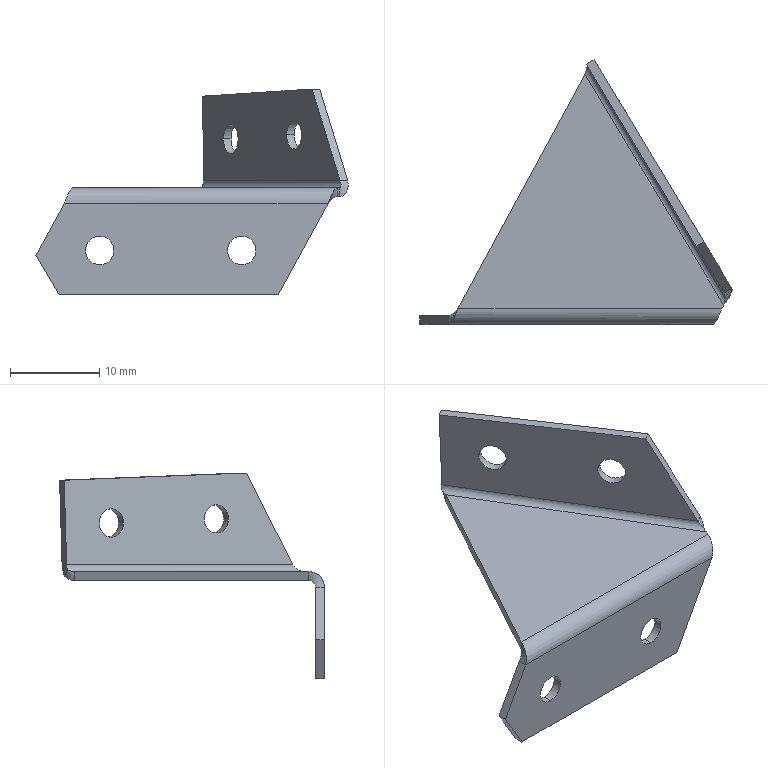Part | SolidWorks | features BaseBody 1 | 1 solid | 32 faces | box 35.031 x 29.701 x 23.105 mm | volume 1039 mm3 | plane 15 | cylinder 12 | spline 5 | commonest cylinder face diameters 3.2 x8 1.5 x2 3.5 x2
STEP:
#1=CARTESIAN_POINT('',(-8.394,13.485,6.933));
#2=VERTEX_POINT('',#1);
#3=CARTESIAN_POINT('',(-6.743,10.744,6.933));
#4=VERTEX_POINT('',#3);
#5=CARTESIAN_POINT('',(-7.568,12.114,6.933));
#6=DIRECTION('',(-0.8566,-0.516,0.));
#7=DIRECTION('',(-0.516,0.8566,0.));
#8=AXIS2_PLACEMENT_3D('',#5,#6,#7);
#9=CIRCLE('',#8,1.6);
#10=EDGE_CURVE('',#2,#4,#9,.T.);
#11=ORIENTED_EDGE('',*,*,#10,.T.);
#12=CARTESIAN_POINT('',(-5.886,11.26,6.933));
#13=VERTEX_POINT('',#12);
#14=CARTESIAN_POINT('',(-6.743,10.744,6.933));
#15=DIRECTION('',(0.8566,0.516,0.));
#16=VECTOR('',#15,1000.);
#17=LINE('',#14,#16);
#18=EDGE_CURVE('',#4,#13,#17,.T.);
#19=ORIENTED_EDGE('',*,*,#18,.T.);
#20=CARTESIAN_POINT('',(-7.537,14.001,6.933));
#21=VERTEX_POINT('',#20);
#22=CARTESIAN_POINT('',(-6.712,12.63,6.933));
#23=DIRECTION('',(0.8566,0.516,0.));
#24=DIRECTION('',(-0.516,0.8566,0.));
#25=AXIS2_PLACEMENT_3D('',#22,#23,#24);
#26=CIRCLE('',#25,1.6);
#27=EDGE_CURVE('',#13,#21,#26,.T.);
#28=ORIENTED_EDGE('',*,*,#27,.T.);
#29=CARTESIAN_POINT('',(-8.394,13.485,6.933));
#30=DIRECTION('',(0.8566,0.516,0.));
#31=VECTOR('',#30,1000.);
#32=LINE('',#29,#31);
#33=EDGE_CURVE('',#2,#21,#32,.T.);
#34=ORIENTED_EDGE('',*,*,#33,.F.);
#35=EDGE_LOOP('',(#11,#19,#28,#34));
#36=FACE_OUTER_BOUND('',#35,.T.);
#37=CARTESIAN_POINT('',(-7.568,12.114,6.933));
#38=DIRECTION('',(0.8566,0.516,0.));
#39=DIRECTION('',(-0.516,0.8566,0.));
#40=AXIS2_PLACEMENT_3D('',#37,#38,#39);
#41=CYLINDRICAL_SURFACE('',#40,1.6);
#42=ADVANCED_FACE('',(#36),#41,.F.);
#43=CARTESIAN_POINT('',(-15.496,25.274,6.468));
#44=VERTEX_POINT('',#43);
#45=CARTESIAN_POINT('',(-13.845,22.533,6.468));
#46=VERTEX_POINT('',#45);
#47=CARTESIAN_POINT('',(-14.671,23.904,6.468));
#48=DIRECTION('',(-0.8566,-0.516,0.));
#49=DIRECTION('',(-0.516,0.8566,0.));
#50=AXIS2_PLACEMENT_3D('',#47,#48,#49);
#51=CIRCLE('',#50,1.6);
#52=EDGE_CURVE('',#44,#46,#51,.T.);
#53=ORIENTED_EDGE('',*,*,#52,.T.);
#54=CARTESIAN_POINT('',(-12.988,23.049,6.468));
#55=VERTEX_POINT('',#54);
#56=CARTESIAN_POINT('',(-13.845,22.533,6.468));
#57=DIRECTION('',(0.8566,0.516,0.));
#58=VECTOR('',#57,1000.);
#59=LINE('',#56,#58);
#60=EDGE_CURVE('',#46,#55,#59,.T.);
#61=ORIENTED_EDGE('',*,*,#60,.T.);
#62=CARTESIAN_POINT('',(-14.64,25.79,6.468));
#63=VERTEX_POINT('',#62);
#64=CARTESIAN_POINT('',(-13.814,24.42,6.468));
#65=DIRECTION('',(-0.8566,-0.516,0.));
#66=DIRECTION('',(-0.516,0.8566,0.));
#67=AXIS2_PLACEMENT_3D('',#64,#65,#66);
#68=CIRCLE('',#67,1.6);
#69=EDGE_CURVE('',#63,#55,#68,.T.);
#70=ORIENTED_EDGE('',*,*,#69,.F.);
#71=CARTESIAN_POINT('',(-15.496,25.274,6.468));
#72=DIRECTION('',(0.8566,0.516,0.));
#73=VECTOR('',#72,1000.);
#74=LINE('',#71,#73);
#75=EDGE_CURVE('',#44,#63,#74,.T.);
#76=ORIENTED_EDGE('',*,*,#75,.F.);
#77=EDGE_LOOP('',(#53,#61,#70,#76));
#78=FACE_OUTER_BOUND('',#77,.T.);
#79=CARTESIAN_POINT('',(-14.671,23.904,6.468));
#80=DIRECTION('',(0.8566,0.516,0.));
#81=DIRECTION('',(-0.516,0.8566,0.));
#82=AXIS2_PLACEMENT_3D('',#79,#80,#81);
#83=CYLINDRICAL_SURFACE('',#82,1.6);
#84=ADVANCED_FACE('',(#78),#83,.F.);
#85=CARTESIAN_POINT('',(-29.376,0.,-4.437));
#86=VERTEX_POINT('',#85);
#87=CARTESIAN_POINT('',(-29.376,0.,-7.637));
#88=VERTEX_POINT('',#87);
#89=CARTESIAN_POINT('',(-29.376,0.,-6.037));
#90=DIRECTION('',(0.,-1.,0.));
#91=DIRECTION('',(0.,0.,1.));
#92=AXIS2_PLACEMENT_3D('',#89,#90,#91);
#93=CIRCLE('',#92,1.6);
#94=EDGE_CURVE('',#86,#88,#93,.T.);
#95=ORIENTED_EDGE('',*,*,#94,.T.);
#96=CARTESIAN_POINT('',(-29.376,1.,-7.637));
#97=VERTEX_POINT('',#96);
#98=CARTESIAN_POINT('',(-29.376,0.,-7.637));
#99=DIRECTION('',(0.,1.,0.));
#100=VECTOR('',#99,1000.);
#101=LINE('',#98,#100);
#102=EDGE_CURVE('',#88,#97,#101,.T.);
#103=ORIENTED_EDGE('',*,*,#102,.T.);
#104=CARTESIAN_POINT('',(-29.376,1.,-4.437));
#105=VERTEX_POINT('',#104);
#106=CARTESIAN_POINT('',(-29.376,1.,-6.037));
#107=DIRECTION('',(0.,-1.,0.));
#108=DIRECTION('',(0.,0.,1.));
#109=AXIS2_PLACEMENT_3D('',#106,#107,#108);
#110=CIRCLE('',#109,1.6);
#111=EDGE_CURVE('',#105,#97,#110,.T.);
#112=ORIENTED_EDGE('',*,*,#111,.F.);
#113=CARTESIAN_POINT('',(-29.376,0.,-4.437));
#114=DIRECTION('',(0.,1.,0.));
#115=VECTOR('',#114,1000.);
#116=LINE('',#113,#115);
#117=EDGE_CURVE('',#86,#105,#116,.T.);
#118=ORIENTED_EDGE('',*,*,#117,.F.);
#119=EDGE_LOOP('',(#95,#103,#112,#118));
#120=FACE_OUTER_BOUND('',#119,.T.);
#121=CARTESIAN_POINT('',(-29.376,0.,-6.037));
#122=DIRECTION('',(0.,1.,0.));
#123=DIRECTION('',(0.,0.,1.));
#124=AXIS2_PLACEMENT_3D('',#121,#122,#123);
#125=CYLINDRICAL_SURFACE('',#124,1.6);
#126=ADVANCED_FACE('',(#120),#125,.F.);
#127=CARTESIAN_POINT('',(-13.445,0.,-4.437));
#128=VERTEX_POINT('',#127);
#129=CARTESIAN_POINT('',(-13.445,0.,-7.637));
#130=VERTEX_POINT('',#129);
#131=CARTESIAN_POINT('',(-13.445,0.,-6.037));
#132=DIRECTION('',(0.,-1.,0.));
#133=DIRECTION('',(0.,0.,1.));
#134=AXIS2_PLACEMENT_3D('',#131,#132,#133);
#135=CIRCLE('',#134,1.6);
#136=EDGE_CURVE('',#128,#130,#135,.T.);
#137=ORIENTED_EDGE('',*,*,#136,.T.);
#138=CARTESIAN_POINT('',(-13.445,1.,-7.637));
#139=VERTEX_POINT('',#138);
#140=CARTESIAN_POINT('',(-13.445,0.,-7.637));
#141=DIRECTION('',(0.,1.,0.));
#142=VECTOR('',#141,1000.);
#143=LINE('',#140,#142);
#144=EDGE_CURVE('',#130,#139,#143,.T.);
#145=ORIENTED_EDGE('',*,*,#144,.T.);
#146=CARTESIAN_POINT('',(-13.445,1.,-4.437));
#147=VERTEX_POINT('',#146);
#148=CARTESIAN_POINT('',(-13.445,1.,-6.037));
#149=DIRECTION('',(0.,-1.,0.));
#150=DIRECTION('',(0.,0.,1.));
#151=AXIS2_PLACEMENT_3D('',#148,#149,#150);
#152=CIRCLE('',#151,1.6);
#153=EDGE_CURVE('',#147,#139,#152,.T.);
#154=ORIENTED_EDGE('',*,*,#153,.F.);
#155=CARTESIAN_POINT('',(-13.445,0.,-4.437));
#156=DIRECTION('',(0.,1.,0.));
#157=VECTOR('',#156,1000.);
#158=LINE('',#155,#157);
#159=EDGE_CURVE('',#128,#147,#158,.T.);
#160=ORIENTED_EDGE('',*,*,#159,.F.);
#161=EDGE_LOOP('',(#137,#145,#154,#160));
#162=FACE_OUTER_BOUND('',#161,.T.);
#163=CARTESIAN_POINT('',(-13.445,0.,-6.037));
#164=DIRECTION('',(0.,1.,0.));
#165=DIRECTION('',(0.,0.,1.));
#166=AXIS2_PLACEMENT_3D('',#163,#164,#165);
#167=CYLINDRICAL_SURFACE('',#166,1.6);
#168=ADVANCED_FACE('',(#162),#167,.F.);
#169=ORIENTED_EDGE('',*,*,#18,.F.);
#170=CARTESIAN_POINT('',(-7.568,12.114,6.933));
#171=DIRECTION('',(-0.8566,-0.516,0.));
#172=DIRECTION('',(-0.516,0.8566,0.));
#173=AXIS2_PLACEMENT_3D('',#170,#171,#172);
#174=CIRCLE('',#173,1.6);
#175=EDGE_CURVE('',#4,#2,#174,.T.);
#176=ORIENTED_EDGE('',*,*,#175,.T.);
#177=ORIENTED_EDGE('',*,*,#33,.T.);
#178=CARTESIAN_POINT('',(-6.712,12.63,6.933));
#179=DIRECTION('',(0.8566,0.516,0.));
#180=DIRECTION('',(-0.516,0.8566,0.));
#181=AXIS2_PLACEMENT_3D('',#178,#179,#180);
#182=CIRCLE('',#181,1.6);
#183=EDGE_CURVE('',#21,#13,#182,.T.);
#184=ORIENTED_EDGE('',*,*,#183,.T.);
#185=EDGE_LOOP('',(#169,#176,#177,#184));
#186=FACE_OUTER_BOUND('',#185,.T.);
#187=CARTESIAN_POINT('',(-7.568,12.114,6.933));
#188=DIRECTION('',(0.8566,0.516,0.));
#189=DIRECTION('',(-0.516,0.8566,0.));
#190=AXIS2_PLACEMENT_3D('',#187,#188,#189);
#191=CYLINDRICAL_SURFACE('',#190,1.6);
#192=ADVANCED_FACE('',(#186),#191,.F.);
#193=ORIENTED_EDGE('',*,*,#69,.T.);
#194=CARTESIAN_POINT('',(-13.814,24.42,6.468));
#195=DIRECTION('',(-0.8566,-0.516,0.));
#196=DIRECTION('',(-0.516,0.8566,0.));
#197=AXIS2_PLACEMENT_3D('',#194,#195,#196);
#198=CIRCLE('',#197,1.6);
#199=EDGE_CURVE('',#55,#63,#198,.T.);
#200=ORIENTED_EDGE('',*,*,#199,.T.);
#201=EDGE_LOOP('',(#193,#200));
#202=FACE_BOUND('',#201,.T.);
#203=ORIENTED_EDGE('',*,*,#183,.F.);
#204=ORIENTED_EDGE('',*,*,#27,.F.);
#205=EDGE_LOOP('',(#203,#204));
#206=FACE_BOUND('',#205,.T.);
#207=CARTESIAN_POINT('',(-16.995,29.701,11.262));
#208=VERTEX_POINT('',#207);
#209=CARTESIAN_POINT('',(-4.678,9.254,12.069));
#210=VERTEX_POINT('',#209);
#211=CARTESIAN_POINT('',(-16.995,29.701,11.262));
#212=DIRECTION('',(0.5157,-0.8561,0.03376));
#213=VECTOR('',#212,1000.);
#214=LINE('',#211,#213);
#215=EDGE_CURVE('',#208,#210,#214,.T.);
#216=ORIENTED_EDGE('',*,*,#215,.T.);
#217=CARTESIAN_POINT('',(-1.55,4.061,1.75));
#218=VERTEX_POINT('',#217);
#219=CARTESIAN_POINT('',(-4.678,9.254,12.069));
#220=DIRECTION('',(0.2614,-0.4339,-0.8622));
#221=VECTOR('',#220,1000.);
#222=LINE('',#219,#221);
#223=EDGE_CURVE('',#210,#218,#222,.T.);
#224=ORIENTED_EDGE('',*,*,#223,.T.);
#225=CARTESIAN_POINT('',(-16.83,29.426,1.75));
#226=VERTEX_POINT('',#225);
#227=CARTESIAN_POINT('',(-1.55,4.061,1.75));
#228=DIRECTION('',(-0.516,0.8566,0.));
#229=VECTOR('',#228,1000.);
#230=LINE('',#227,#229);
#231=EDGE_CURVE('',#218,#226,#230,.T.);
#232=ORIENTED_EDGE('',*,*,#231,.T.);
#233=CARTESIAN_POINT('',(-16.83,29.426,1.75));
#234=DIRECTION('',(-0.01742,0.02892,0.9994));
#235=VECTOR('',#234,1000.);
#236=LINE('',#233,#235);
#237=EDGE_CURVE('',#226,#208,#236,.T.);
#238=ORIENTED_EDGE('',*,*,#237,.T.);
#239=EDGE_LOOP('',(#216,#224,#232,#238));
#240=FACE_OUTER_BOUND('',#239,.T.);
#241=CARTESIAN_POINT('',(-19.235,33.419,4.412));
#242=DIRECTION('',(0.8566,0.516,0.));
#243=DIRECTION('',(0.2663,-0.442,0.8566));
#244=AXIS2_PLACEMENT_3D('',#241,#242,#243);
#245=PLANE('',#244);
#246=ADVANCED_FACE('',(#202,#206,#240),#245,.T.);
#247=ORIENTED_EDGE('',*,*,#52,.F.);
#248=CARTESIAN_POINT('',(-14.671,23.904,6.468));
#249=DIRECTION('',(-0.8566,-0.516,0.));
#250=DIRECTION('',(-0.516,0.8566,0.));
#251=AXIS2_PLACEMENT_3D('',#248,#249,#250);
#252=CIRCLE('',#251,1.6);
#253=EDGE_CURVE('',#46,#44,#252,.T.);
#254=ORIENTED_EDGE('',*,*,#253,.F.);
#255=EDGE_LOOP('',(#247,#254));
#256=FACE_BOUND('',#255,.T.);
#257=ORIENTED_EDGE('',*,*,#10,.F.);
#258=ORIENTED_EDGE('',*,*,#175,.F.);
#259=EDGE_LOOP('',(#257,#258));
#260=FACE_BOUND('',#259,.T.);
#261=CARTESIAN_POINT('',(-17.852,29.185,11.262));
#262=VERTEX_POINT('',#261);
#263=CARTESIAN_POINT('',(-5.534,8.738,12.069));
#264=VERTEX_POINT('',#263);
#265=CARTESIAN_POINT('',(-5.534,8.738,12.069));
#266=DIRECTION('',(0.5157,-0.8561,0.03376));
#267=VECTOR('',#266,1000.);
#268=LINE('',#265,#267);
#269=EDGE_CURVE('',#262,#264,#268,.T.);
#270=ORIENTED_EDGE('',*,*,#269,.F.);
#271=CARTESIAN_POINT('',(-17.686,28.91,1.75));
#272=VERTEX_POINT('',#271);
#273=CARTESIAN_POINT('',(-17.852,29.185,11.262));
#274=DIRECTION('',(-0.01742,0.02892,0.9994));
#275=VECTOR('',#274,1000.);
#276=LINE('',#273,#275);
#277=EDGE_CURVE('',#272,#262,#276,.T.);
#278=ORIENTED_EDGE('',*,*,#277,.F.);
#279=CARTESIAN_POINT('',(-2.406,3.545,1.75));
#280=VERTEX_POINT('',#279);
#281=CARTESIAN_POINT('',(-17.782,29.068,1.75));
#282=DIRECTION('',(-0.516,0.8566,0.));
#283=VECTOR('',#282,1000.);
#284=LINE('',#281,#283);
#285=EDGE_CURVE('',#280,#272,#284,.T.);
#286=ORIENTED_EDGE('',*,*,#285,.F.);
#287=CARTESIAN_POINT('',(-2.406,3.545,1.75));
#288=DIRECTION('',(0.2614,-0.4339,-0.8622));
#289=VECTOR('',#288,1000.);
#290=LINE('',#287,#289);
#291=EDGE_CURVE('',#264,#280,#290,.T.);
#292=ORIENTED_EDGE('',*,*,#291,.F.);
#293=EDGE_LOOP('',(#270,#278,#286,#292));
#294=FACE_OUTER_BOUND('',#293,.T.);
#295=CARTESIAN_POINT('',(-20.092,32.903,4.412));
#296=DIRECTION('',(0.8566,0.516,0.));
#297=DIRECTION('',(0.2663,-0.442,0.8566));
#298=AXIS2_PLACEMENT_3D('',#295,#296,#297);
#299=PLANE('',#298);
#300=ADVANCED_FACE('',(#256,#260,#294),#299,.F.);
#301=ORIENTED_EDGE('',*,*,#60,.F.);
#302=ORIENTED_EDGE('',*,*,#253,.T.);
#303=ORIENTED_EDGE('',*,*,#75,.T.);
#304=ORIENTED_EDGE('',*,*,#199,.F.);
#305=EDGE_LOOP('',(#301,#302,#303,#304));
#306=FACE_OUTER_BOUND('',#305,.T.);
#307=CARTESIAN_POINT('',(-14.671,23.904,6.468));
#308=DIRECTION('',(0.8566,0.516,0.));
#309=DIRECTION('',(-0.516,0.8566,0.));
#310=AXIS2_PLACEMENT_3D('',#307,#308,#309);
#311=CYLINDRICAL_SURFACE('',#310,1.6);
#312=ADVANCED_FACE('',(#306),#311,.F.);
#313=CARTESIAN_POINT('',(-5.106,8.996,12.069));
#314=DIRECTION('',(-0.8566,-0.516,0.));
#315=VECTOR('',#314,1000.);
#316=LINE('',#313,#315);
#317=EDGE_CURVE('',#210,#264,#316,.T.);
#318=ORIENTED_EDGE('',*,*,#317,.T.);
#319=ORIENTED_EDGE('',*,*,#291,.T.);
#320=CARTESIAN_POINT('',(-1.978,3.803,1.75));
#321=DIRECTION('',(-0.8566,-0.516,0.));
#322=VECTOR('',#321,1000.);
#323=LINE('',#320,#322);
#324=EDGE_CURVE('',#218,#280,#323,.T.);
#325=ORIENTED_EDGE('',*,*,#324,.F.);
#326=ORIENTED_EDGE('',*,*,#223,.F.);
#327=EDGE_LOOP('',(#318,#319,#325,#326));
#328=FACE_OUTER_BOUND('',#327,.T.);
#329=CARTESIAN_POINT('',(-1.55,4.061,1.75));
#330=DIRECTION('',(0.4449,-0.7385,0.5066));
#331=DIRECTION('',(-0.2614,0.4339,0.8622));
#332=AXIS2_PLACEMENT_3D('',#329,#330,#331);
#333=PLANE('',#332);
#334=ADVANCED_FACE('',(#328),#333,.T.);
#335=ORIENTED_EDGE('',*,*,#269,.T.);
#336=ORIENTED_EDGE('',*,*,#317,.F.);
#337=ORIENTED_EDGE('',*,*,#215,.F.);
#338=CARTESIAN_POINT('',(-17.424,29.443,11.262));
#339=DIRECTION('',(-0.8566,-0.516,0.));
#340=VECTOR('',#339,1000.);
#341=LINE('',#338,#340);
#342=EDGE_CURVE('',#208,#262,#341,.T.);
#343=ORIENTED_EDGE('',*,*,#342,.T.);
#344=EDGE_LOOP('',(#335,#336,#337,#343));
#345=FACE_OUTER_BOUND('',#344,.T.);
#346=CARTESIAN_POINT('',(-4.678,9.254,12.069));
#347=DIRECTION('',(-0.01742,0.02892,0.9994));
#348=DIRECTION('',(-0.5157,0.8561,-0.03376));
#349=AXIS2_PLACEMENT_3D('',#346,#347,#348);
#350=PLANE('',#349);
#351=ADVANCED_FACE('',(#345),#350,.T.);
#352=ORIENTED_EDGE('',*,*,#342,.F.);
#353=ORIENTED_EDGE('',*,*,#237,.F.);
#354=CARTESIAN_POINT('',(-17.258,29.168,1.75));
#355=DIRECTION('',(-0.8566,-0.516,0.));
#356=VECTOR('',#355,1000.);
#357=LINE('',#354,#356);
#358=EDGE_CURVE('',#226,#272,#357,.T.);
#359=ORIENTED_EDGE('',*,*,#358,.T.);
#360=ORIENTED_EDGE('',*,*,#277,.T.);
#361=EDGE_LOOP('',(#352,#353,#359,#360));
#362=FACE_OUTER_BOUND('',#361,.T.);
#363=CARTESIAN_POINT('',(-16.995,29.701,11.262));
#364=DIRECTION('',(-0.5157,0.8561,-0.03376));
#365=DIRECTION('',(0.01742,-0.02892,-0.9994));
#366=AXIS2_PLACEMENT_3D('',#363,#364,#365);
#367=PLANE('',#366);
#368=ADVANCED_FACE('',(#362),#367,.T.);
#369=ORIENTED_EDGE('',*,*,#231,.F.);
#370=CARTESIAN_POINT('',(-2.453,2.17,0.));
#371=VERTEX_POINT('',#370);
#372=CARTESIAN_POINT('',(-2.453,2.17,0.));
#373=CARTESIAN_POINT('',(-2.305,2.372,0.));
#374=CARTESIAN_POINT('',(-2.161,2.57,0.04509));
#375=CARTESIAN_POINT('',(-1.962,2.859,0.1772));
#376=CARTESIAN_POINT('',(-1.901,2.952,0.2311));
#377=CARTESIAN_POINT('',(-1.788,3.131,0.3577));
#378=CARTESIAN_POINT('',(-1.736,3.219,0.4312));
#379=CARTESIAN_POINT('',(-1.647,3.386,0.5935));
#380=CARTESIAN_POINT('',(-1.609,3.464,0.6817));
#381=CARTESIAN_POINT('',(-1.55,3.611,0.8714));
#382=CARTESIAN_POINT('',(-1.528,3.681,0.974));
#383=CARTESIAN_POINT('',(-1.489,3.873,1.291));
#384=CARTESIAN_POINT('',(-1.5,3.978,1.519));
#385=CARTESIAN_POINT('',(-1.55,4.061,1.75));
#386=B_SPLINE_CURVE_WITH_KNOTS('',3,(#372,#373,#374,#375,#376,#377,#378,#379,#380,#381,#382,#383,#384,#385),.UNSPECIFIED.,.F.,.F.,(4,2,2,2,2,2,4),(0.,0.0007413,0.001112,0.001483,0.001853,0.002224,0.002965),.UNSPECIFIED.);
#387=EDGE_CURVE('',#371,#218,#386,.T.);
#388=ORIENTED_EDGE('',*,*,#387,.F.);
#389=CARTESIAN_POINT('',(-18.014,28.,0.));
#390=VERTEX_POINT('',#389);
#391=CARTESIAN_POINT('',(-10.391,15.346,0.));
#392=DIRECTION('',(0.516,-0.8566,0.));
#393=VECTOR('',#392,1000.);
#394=LINE('',#391,#393);
#395=EDGE_CURVE('',#390,#371,#394,.T.);
#396=ORIENTED_EDGE('',*,*,#395,.F.);
#397=CARTESIAN_POINT('',(-17.252,29.133,0.5126));
#398=VERTEX_POINT('',#397);
#399=CARTESIAN_POINT('',(-17.252,29.133,0.5126));
#400=CARTESIAN_POINT('',(-17.342,28.965,0.3491));
#401=CARTESIAN_POINT('',(-17.457,28.785,0.2214));
#402=CARTESIAN_POINT('',(-17.721,28.4,0.04513));
#403=CARTESIAN_POINT('',(-17.866,28.203,0.));
#404=CARTESIAN_POINT('',(-18.014,28.,0.));
#405=B_SPLINE_CURVE_WITH_KNOTS('',3,(#399,#400,#401,#402,#403,#404),.UNSPECIFIED.,.F.,.F.,(4,2,4),(0.,0.0007413,0.001483),.UNSPECIFIED.);
#406=EDGE_CURVE('',#398,#390,#405,.T.);
#407=ORIENTED_EDGE('',*,*,#406,.F.);
#408=CARTESIAN_POINT('',(-16.83,29.426,1.75));
#409=CARTESIAN_POINT('',(-16.827,29.421,1.521));
#410=CARTESIAN_POINT('',(-16.863,29.393,1.292));
#411=CARTESIAN_POINT('',(-17.007,29.293,0.8687));
#412=CARTESIAN_POINT('',(-17.116,29.221,0.6745));
#413=CARTESIAN_POINT('',(-17.252,29.133,0.5126));
#414=B_SPLINE_CURVE_WITH_KNOTS('',3,(#408,#409,#410,#411,#412,#413),.UNSPECIFIED.,.F.,.F.,(4,2,4),(0.,0.5,1.),.UNSPECIFIED.);
#415=EDGE_CURVE('',#226,#398,#414,.T.);
#416=ORIENTED_EDGE('',*,*,#415,.F.);
#417=EDGE_LOOP('',(#369,#388,#396,#407,#416));
#418=FACE_OUTER_BOUND('',#417,.T.);
#419=CARTESIAN_POINT('',(-18.424,28.681,1.75));
#420=DIRECTION('',(0.516,-0.8566,0.));
#421=DIRECTION('',(0.8566,0.516,0.));
#422=AXIS2_PLACEMENT_3D('',#419,#420,#421);
#423=CYLINDRICAL_SURFACE('',#422,1.75);
#424=ADVANCED_FACE('',(#418),#423,.T.);
#425=CARTESIAN_POINT('',(-2.453,2.17,1.));
#426=VERTEX_POINT('',#425);
#427=CARTESIAN_POINT('',(-2.453,2.17,1.));
#428=CARTESIAN_POINT('',(-2.419,2.304,1.));
#429=CARTESIAN_POINT('',(-2.385,2.435,1.019));
#430=CARTESIAN_POINT('',(-2.328,2.694,1.094));
#431=CARTESIAN_POINT('',(-2.307,2.819,1.15));
#432=CARTESIAN_POINT('',(-2.287,3.055,1.288));
#433=CARTESIAN_POINT('',(-2.289,3.167,1.372));
#434=CARTESIAN_POINT('',(-2.323,3.369,1.553));
#435=CARTESIAN_POINT('',(-2.356,3.462,1.651));
#436=CARTESIAN_POINT('',(-2.406,3.545,1.75));
#437=B_SPLINE_CURVE_WITH_KNOTS('',3,(#427,#428,#429,#430,#431,#432,#433,#434,#435,#436),.UNSPECIFIED.,.F.,.F.,(4,2,2,2,4),(0.,0.0004099,0.0008199,0.00123,0.00164),.UNSPECIFIED.);
#438=EDGE_CURVE('',#426,#280,#437,.T.);
#439=ORIENTED_EDGE('',*,*,#438,.T.);
#440=ORIENTED_EDGE('',*,*,#285,.T.);
#441=CARTESIAN_POINT('',(-17.857,28.768,1.22));
#442=VERTEX_POINT('',#441);
#443=CARTESIAN_POINT('',(-17.686,28.91,1.75));
#444=CARTESIAN_POINT('',(-17.681,28.9,1.554));
#445=CARTESIAN_POINT('',(-17.744,28.849,1.359));
#446=CARTESIAN_POINT('',(-17.857,28.768,1.22));
#447=B_SPLINE_CURVE_WITH_KNOTS('',3,(#443,#444,#445,#446),.UNSPECIFIED.,.F.,.F.,(4,4),(0.,1.),.UNSPECIFIED.);
#448=EDGE_CURVE('',#272,#442,#447,.T.);
#449=ORIENTED_EDGE('',*,*,#448,.T.);
#450=CARTESIAN_POINT('',(-18.014,28.,1.));
#451=VERTEX_POINT('',#450);
#452=CARTESIAN_POINT('',(-17.857,28.768,1.22));
#453=CARTESIAN_POINT('',(-17.877,28.531,1.08));
#454=CARTESIAN_POINT('',(-17.945,28.267,1.));
#455=CARTESIAN_POINT('',(-18.014,28.,1.));
#456=B_SPLINE_CURVE_WITH_KNOTS('',3,(#452,#453,#454,#455),.UNSPECIFIED.,.F.,.F.,(4,4),(0.,0.0008241),.UNSPECIFIED.);
#457=EDGE_CURVE('',#442,#451,#456,.T.);
#458=ORIENTED_EDGE('',*,*,#457,.T.);
#459=CARTESIAN_POINT('',(-10.391,15.346,1.));
#460=DIRECTION('',(0.516,-0.8566,0.));
#461=VECTOR('',#460,1000.);
#462=LINE('',#459,#461);
#463=EDGE_CURVE('',#451,#426,#462,.T.);
#464=ORIENTED_EDGE('',*,*,#463,.T.);
#465=EDGE_LOOP('',(#439,#440,#449,#458,#464));
#466=FACE_OUTER_BOUND('',#465,.T.);
#467=CARTESIAN_POINT('',(-18.424,28.681,1.75));
#468=DIRECTION('',(0.516,-0.8566,0.));
#469=DIRECTION('',(0.8566,0.516,0.));
#470=AXIS2_PLACEMENT_3D('',#467,#468,#469);
#471=CYLINDRICAL_SURFACE('',#470,0.75);
#472=ADVANCED_FACE('',(#466),#471,.F.);
#473=ORIENTED_EDGE('',*,*,#358,.F.);
#474=ORIENTED_EDGE('',*,*,#415,.T.);
#475=CARTESIAN_POINT('',(-17.554,28.95,0.8661));
#476=DIRECTION('',(-0.6057,-0.3649,0.7071));
#477=VECTOR('',#476,1000.);
#478=LINE('',#475,#477);
#479=EDGE_CURVE('',#398,#442,#478,.T.);
#480=ORIENTED_EDGE('',*,*,#479,.T.);
#481=ORIENTED_EDGE('',*,*,#448,.F.);
#482=EDGE_LOOP('',(#473,#474,#480,#481));
#483=FACE_OUTER_BOUND('',#482,.T.);
#484=CARTESIAN_POINT('',(-17.246,29.137,0.5055));
#485=CARTESIAN_POINT('',(-17.109,29.225,0.6684));
#486=CARTESIAN_POINT('',(-17.,29.297,0.8636));
#487=CARTESIAN_POINT('',(-16.855,29.398,1.289));
#488=CARTESIAN_POINT('',(-16.818,29.426,1.52));
#489=CARTESIAN_POINT('',(-16.821,29.431,1.75));
#490=CARTESIAN_POINT('',(-17.252,29.133,0.5126));
#491=CARTESIAN_POINT('',(-17.116,29.221,0.6746));
#492=CARTESIAN_POINT('',(-17.007,29.293,0.8687));
#493=CARTESIAN_POINT('',(-16.863,29.393,1.292));
#494=CARTESIAN_POINT('',(-16.827,29.421,1.521));
#495=CARTESIAN_POINT('',(-16.83,29.426,1.75));
#496=CARTESIAN_POINT('',(-17.857,28.768,1.22));
#497=CARTESIAN_POINT('',(-17.801,28.809,1.289));
#498=CARTESIAN_POINT('',(-17.756,28.842,1.372));
#499=CARTESIAN_POINT('',(-17.697,28.89,1.554));
#500=CARTESIAN_POINT('',(-17.683,28.905,1.652));
#501=CARTESIAN_POINT('',(-17.686,28.91,1.75));
#502=CARTESIAN_POINT('',(-17.863,28.764,1.227));
#503=CARTESIAN_POINT('',(-17.808,28.804,1.295));
#504=CARTESIAN_POINT('',(-17.764,28.837,1.377));
#505=CARTESIAN_POINT('',(-17.706,28.885,1.556));
#506=CARTESIAN_POINT('',(-17.692,28.9,1.653));
#507=CARTESIAN_POINT('',(-17.695,28.905,1.75));
#508=B_SPLINE_SURFACE_WITH_KNOTS('',1,3,((#484,#485,#486,#487,#488,#489),(#490,#491,#492,#493,#494,#495),(#496,#497,#498,#499,#500,#501),(#502,#503,#504,#505,#506,#507)),.UNSPECIFIED.,.F.,.F.,.F.,(2,1,1,2),(4,2,4),(-0.01,0.,1.,1.01),(0.,0.5,1.),.UNSPECIFIED.);
#509=ADVANCED_FACE('',(#483),#508,.T.);
#510=CARTESIAN_POINT('',(-2.453,2.17,0.5));
#511=DIRECTION('',(0.,0.,-1.));
#512=VECTOR('',#511,1000.);
#513=LINE('',#510,#512);
#514=EDGE_CURVE('',#426,#371,#513,.T.);
#515=ORIENTED_EDGE('',*,*,#514,.T.);
#516=ORIENTED_EDGE('',*,*,#387,.T.);
#517=ORIENTED_EDGE('',*,*,#324,.T.);
#518=ORIENTED_EDGE('',*,*,#438,.F.);
#519=EDGE_LOOP('',(#515,#516,#517,#518));
#520=FACE_OUTER_BOUND('',#519,.T.);
#521=CARTESIAN_POINT('',(-1.541,4.066,1.75));
#522=CARTESIAN_POINT('',(-1.491,3.984,1.52));
#523=CARTESIAN_POINT('',(-1.481,3.878,1.289));
#524=CARTESIAN_POINT('',(-1.533,3.622,0.8636));
#525=CARTESIAN_POINT('',(-1.595,3.473,0.6684));
#526=CARTESIAN_POINT('',(-1.775,3.14,0.3426));
#527=CARTESIAN_POINT('',(-1.893,2.957,0.2121));
#528=CARTESIAN_POINT('',(-2.158,2.572,0.03581));
#529=CARTESIAN_POINT('',(-2.306,2.371,-0.01));
#530=CARTESIAN_POINT('',(-2.453,2.17,-0.01));
#531=CARTESIAN_POINT('',(-1.55,4.061,1.75));
#532=CARTESIAN_POINT('',(-1.5,3.979,1.521));
#533=CARTESIAN_POINT('',(-1.489,3.873,1.292));
#534=CARTESIAN_POINT('',(-1.54,3.618,0.8687));
#535=CARTESIAN_POINT('',(-1.602,3.469,0.6745));
#536=CARTESIAN_POINT('',(-1.78,3.137,0.3506));
#537=CARTESIAN_POINT('',(-1.897,2.954,0.2209));
#538=CARTESIAN_POINT('',(-2.16,2.571,0.04555));
#539=CARTESIAN_POINT('',(-2.307,2.371,0.));
#540=CARTESIAN_POINT('',(-2.453,2.17,0.));
#541=CARTESIAN_POINT('',(-2.406,3.545,1.75));
#542=CARTESIAN_POINT('',(-2.357,3.463,1.652));
#543=CARTESIAN_POINT('',(-2.324,3.37,1.554));
#544=CARTESIAN_POINT('',(-2.289,3.167,1.372));
#545=CARTESIAN_POINT('',(-2.287,3.056,1.289));
#546=CARTESIAN_POINT('',(-2.307,2.82,1.15));
#547=CARTESIAN_POINT('',(-2.328,2.694,1.095));
#548=CARTESIAN_POINT('',(-2.384,2.436,1.02));
#549=CARTESIAN_POINT('',(-2.419,2.303,1.));
#550=CARTESIAN_POINT('',(-2.453,2.17,1.));
#551=CARTESIAN_POINT('',(-2.415,3.54,1.75));
#552=CARTESIAN_POINT('',(-2.365,3.458,1.653));
#553=CARTESIAN_POINT('',(-2.332,3.365,1.556));
#554=CARTESIAN_POINT('',(-2.296,3.162,1.377));
#555=CARTESIAN_POINT('',(-2.294,3.052,1.295));
#556=CARTESIAN_POINT('',(-2.312,2.816,1.158));
#557=CARTESIAN_POINT('',(-2.333,2.692,1.103));
#558=CARTESIAN_POINT('',(-2.387,2.435,1.029));
#559=CARTESIAN_POINT('',(-2.42,2.302,1.01));
#560=CARTESIAN_POINT('',(-2.453,2.17,1.01));
#561=B_SPLINE_SURFACE_WITH_KNOTS('',1,3,((#521,#522,#523,#524,#525,#526,#527,#528,#529,#530),(#531,#532,#533,#534,#535,#536,#537,#538,#539,#540),(#541,#542,#543,#544,#545,#546,#547,#548,#549,#550),(#551,#552,#553,#554,#555,#556,#557,#558,#559,#560)),.UNSPECIFIED.,.F.,.F.,.F.,(2,1,1,2),(4,2,2,2,4),(-0.01,0.,1.,1.01),(0.,0.25,0.5,0.75,1.),.UNSPECIFIED.);
#562=ADVANCED_FACE('',(#520),#561,.T.);
#563=CARTESIAN_POINT('',(-32.267,1.75,0.));
#564=VERTEX_POINT('',#563);
#565=CARTESIAN_POINT('',(-32.267,1.75,0.));
#566=DIRECTION('',(0.4772,0.8788,0.));
#567=VECTOR('',#566,1000.);
#568=LINE('',#565,#567);
#569=EDGE_CURVE('',#564,#390,#568,.T.);
#570=ORIENTED_EDGE('',*,*,#569,.T.);
#571=ORIENTED_EDGE('',*,*,#395,.T.);
#572=CARTESIAN_POINT('',(-2.681,1.75,0.));
#573=VERTEX_POINT('',#572);
#574=CARTESIAN_POINT('',(-2.453,2.17,0.));
#575=DIRECTION('',(-0.4772,-0.8788,0.));
#576=VECTOR('',#575,1000.);
#577=LINE('',#574,#576);
#578=EDGE_CURVE('',#371,#573,#577,.T.);
#579=ORIENTED_EDGE('',*,*,#578,.T.);
#580=CARTESIAN_POINT('',(-17.36,1.75,0.));
#581=DIRECTION('',(-1.,0.,0.));
#582=VECTOR('',#581,1000.);
#583=LINE('',#580,#582);
#584=EDGE_CURVE('',#573,#564,#583,.T.);
#585=ORIENTED_EDGE('',*,*,#584,.T.);
#586=EDGE_LOOP('',(#570,#571,#579,#585));
#587=FACE_OUTER_BOUND('',#586,.T.);
#588=CARTESIAN_POINT('',(-32.446,28.158,0.));
#589=DIRECTION('',(0.,0.,-1.));
#590=DIRECTION('',(1.,0.,0.));
#591=AXIS2_PLACEMENT_3D('',#588,#589,#590);
#592=PLANE('',#591);
#593=ADVANCED_FACE('',(#587),#592,.T.);
#594=ORIENTED_EDGE('',*,*,#479,.F.);
#595=ORIENTED_EDGE('',*,*,#406,.T.);
#596=CARTESIAN_POINT('',(-18.014,28.,0.5));
#597=DIRECTION('',(0.,0.,1.));
#598=VECTOR('',#597,1000.);
#599=LINE('',#596,#598);
#600=EDGE_CURVE('',#390,#451,#599,.T.);
#601=ORIENTED_EDGE('',*,*,#600,.T.);
#602=ORIENTED_EDGE('',*,*,#457,.F.);
#603=EDGE_LOOP('',(#594,#595,#601,#602));
#604=FACE_OUTER_BOUND('',#603,.T.);
#605=CARTESIAN_POINT('',(-18.014,28.,-0.01));
#606=CARTESIAN_POINT('',(-17.866,28.202,-0.01));
#607=CARTESIAN_POINT('',(-17.719,28.403,0.03581));
#608=CARTESIAN_POINT('',(-17.453,28.787,0.2121));
#609=CARTESIAN_POINT('',(-17.336,28.97,0.3426));
#610=CARTESIAN_POINT('',(-17.246,29.137,0.5055));
#611=CARTESIAN_POINT('',(-18.014,28.,0.));
#612=CARTESIAN_POINT('',(-17.867,28.201,0.));
#613=CARTESIAN_POINT('',(-17.721,28.401,0.04555));
#614=CARTESIAN_POINT('',(-17.457,28.784,0.2209));
#615=CARTESIAN_POINT('',(-17.341,28.967,0.3506));
#616=CARTESIAN_POINT('',(-17.252,29.133,0.5126));
#617=CARTESIAN_POINT('',(-18.014,28.,1.));
#618=CARTESIAN_POINT('',(-17.979,28.133,1.));
#619=CARTESIAN_POINT('',(-17.945,28.266,1.02));
#620=CARTESIAN_POINT('',(-17.889,28.525,1.095));
#621=CARTESIAN_POINT('',(-17.867,28.65,1.15));
#622=CARTESIAN_POINT('',(-17.857,28.768,1.22));
#623=CARTESIAN_POINT('',(-18.014,28.,1.01));
#624=CARTESIAN_POINT('',(-17.981,28.133,1.01));
#625=CARTESIAN_POINT('',(-17.947,28.265,1.029));
#626=CARTESIAN_POINT('',(-17.893,28.522,1.103));
#627=CARTESIAN_POINT('',(-17.872,28.647,1.158));
#628=CARTESIAN_POINT('',(-17.863,28.764,1.227));
#629=B_SPLINE_SURFACE_WITH_KNOTS('',1,3,((#605,#606,#607,#608,#609,#610),(#611,#612,#613,#614,#615,#616),(#617,#618,#619,#620,#621,#622),(#623,#624,#625,#626,#627,#628)),.UNSPECIFIED.,.F.,.F.,.F.,(2,1,1,2),(4,2,4),(-0.01,0.,1.,1.01),(0.,0.5,1.),.UNSPECIFIED.);
#630=ADVANCED_FACE('',(#604),#629,.T.);
#631=CARTESIAN_POINT('',(-32.267,1.75,1.));
#632=VERTEX_POINT('',#631);
#633=CARTESIAN_POINT('',(-18.014,28.,1.));
#634=DIRECTION('',(0.4772,0.8788,0.));
#635=VECTOR('',#634,1000.);
#636=LINE('',#633,#635);
#637=EDGE_CURVE('',#632,#451,#636,.T.);
#638=ORIENTED_EDGE('',*,*,#637,.F.);
#639=CARTESIAN_POINT('',(-2.681,1.75,1.));
#640=VERTEX_POINT('',#639);
#641=CARTESIAN_POINT('',(-17.36,1.75,1.));
#642=DIRECTION('',(-1.,0.,0.));
#643=VECTOR('',#642,1000.);
#644=LINE('',#641,#643);
#645=EDGE_CURVE('',#640,#632,#644,.T.);
#646=ORIENTED_EDGE('',*,*,#645,.F.);
#647=CARTESIAN_POINT('',(-2.681,1.75,1.));
#648=DIRECTION('',(-0.4772,-0.8788,0.));
#649=VECTOR('',#648,1000.);
#650=LINE('',#647,#649);
#651=EDGE_CURVE('',#426,#640,#650,.T.);
#652=ORIENTED_EDGE('',*,*,#651,.F.);
#653=ORIENTED_EDGE('',*,*,#463,.F.);
#654=EDGE_LOOP('',(#638,#646,#652,#653));
#655=FACE_OUTER_BOUND('',#654,.T.);
#656=CARTESIAN_POINT('',(-32.446,28.158,1.));
#657=DIRECTION('',(0.,0.,-1.));
#658=DIRECTION('',(1.,0.,0.));
#659=AXIS2_PLACEMENT_3D('',#656,#657,#658);
#660=PLANE('',#659);
#661=ADVANCED_FACE('',(#655),#660,.F.);
#662=ORIENTED_EDGE('',*,*,#578,.F.);
#663=ORIENTED_EDGE('',*,*,#514,.F.);
#664=ORIENTED_EDGE('',*,*,#651,.T.);
#665=CARTESIAN_POINT('',(-2.681,1.75,0.5));
#666=DIRECTION('',(0.,0.,-1.));
#667=VECTOR('',#666,1000.);
#668=LINE('',#665,#667);
#669=EDGE_CURVE('',#640,#573,#668,.T.);
#670=ORIENTED_EDGE('',*,*,#669,.T.);
#671=EDGE_LOOP('',(#662,#663,#664,#670));
#672=FACE_OUTER_BOUND('',#671,.T.);
#673=CARTESIAN_POINT('',(-2.681,1.75,0.));
#674=DIRECTION('',(0.8788,-0.4772,0.));
#675=DIRECTION('',(0.4772,0.8788,0.));
#676=AXIS2_PLACEMENT_3D('',#673,#674,#675);
#677=PLANE('',#676);
#678=ADVANCED_FACE('',(#672),#677,.T.);
#679=ORIENTED_EDGE('',*,*,#637,.T.);
#680=ORIENTED_EDGE('',*,*,#600,.F.);
#681=ORIENTED_EDGE('',*,*,#569,.F.);
#682=CARTESIAN_POINT('',(-32.267,1.75,0.5));
#683=DIRECTION('',(0.,0.,1.));
#684=VECTOR('',#683,1000.);
#685=LINE('',#682,#684);
#686=EDGE_CURVE('',#564,#632,#685,.T.);
#687=ORIENTED_EDGE('',*,*,#686,.T.);
#688=EDGE_LOOP('',(#679,#680,#681,#687));
#689=FACE_OUTER_BOUND('',#688,.T.);
#690=CARTESIAN_POINT('',(-18.014,28.,0.));
#691=DIRECTION('',(-0.8788,0.4772,0.));
#692=DIRECTION('',(-0.4772,-0.8788,0.));
#693=AXIS2_PLACEMENT_3D('',#690,#691,#692);
#694=PLANE('',#693);
#695=ADVANCED_FACE('',(#689),#694,.T.);
#696=CARTESIAN_POINT('',(-3.748,1.,-0.75));
#697=VERTEX_POINT('',#696);
#698=CARTESIAN_POINT('',(-2.681,1.75,0.));
#699=CARTESIAN_POINT('',(-2.861,1.552,-0.000000001));
#700=CARTESIAN_POINT('',(-3.036,1.359,-0.08026));
#701=CARTESIAN_POINT('',(-3.392,1.081,-0.3585));
#702=CARTESIAN_POINT('',(-3.569,1.,-0.5521));
#703=CARTESIAN_POINT('',(-3.748,1.,-0.75));
#704=B_SPLINE_CURVE_WITH_KNOTS('',3,(#698,#699,#700,#701,#702,#703),.UNSPECIFIED.,.F.,.F.,(4,2,4),(0.,0.0007929,0.001586),.UNSPECIFIED.);
#705=EDGE_CURVE('',#573,#697,#704,.T.);
#706=ORIENTED_EDGE('',*,*,#705,.T.);
#707=CARTESIAN_POINT('',(-33.333,1.,-0.75));
#708=VERTEX_POINT('',#707);
#709=CARTESIAN_POINT('',(-18.007,1.,-0.75));
#710=DIRECTION('',(-1.,0.,0.));
#711=VECTOR('',#710,1000.);
#712=LINE('',#709,#711);
#713=EDGE_CURVE('',#697,#708,#712,.T.);
#714=ORIENTED_EDGE('',*,*,#713,.T.);
#715=CARTESIAN_POINT('',(-33.333,1.,-0.75));
#716=CARTESIAN_POINT('',(-33.154,1.,-0.5521));
#717=CARTESIAN_POINT('',(-32.978,1.08,-0.3592));
#718=CARTESIAN_POINT('',(-32.622,1.358,-0.0807));
#719=CARTESIAN_POINT('',(-32.446,1.552,0.));
#720=CARTESIAN_POINT('',(-32.267,1.75,0.));
#721=B_SPLINE_CURVE_WITH_KNOTS('',3,(#715,#716,#717,#718,#719,#720),.UNSPECIFIED.,.F.,.F.,(4,2,4),(0.,0.0007929,0.001586),.UNSPECIFIED.);
#722=EDGE_CURVE('',#708,#564,#721,.T.);
#723=ORIENTED_EDGE('',*,*,#722,.T.);
#724=ORIENTED_EDGE('',*,*,#584,.F.);
#725=EDGE_LOOP('',(#706,#714,#723,#724));
#726=FACE_OUTER_BOUND('',#725,.T.);
#727=CARTESIAN_POINT('',(-2.498,1.75,-0.75));
#728=DIRECTION('',(-1.,0.,0.));
#729=DIRECTION('',(0.,0.,1.));
#730=AXIS2_PLACEMENT_3D('',#727,#728,#729);
#731=CYLINDRICAL_SURFACE('',#730,0.75);
#732=ADVANCED_FACE('',(#726),#731,.F.);
#733=CARTESIAN_POINT('',(-3.748,0.,-0.75));
#734=VERTEX_POINT('',#733);
#735=CARTESIAN_POINT('',(-33.333,0.,-0.75));
#736=VERTEX_POINT('',#735);
#737=CARTESIAN_POINT('',(-18.007,0.,-0.75));
#738=DIRECTION('',(-1.,0.,0.));
#739=VECTOR('',#738,1000.);
#740=LINE('',#737,#739);
#741=EDGE_CURVE('',#734,#736,#740,.T.);
#742=ORIENTED_EDGE('',*,*,#741,.F.);
#743=CARTESIAN_POINT('',(-2.681,1.75,1.));
#744=CARTESIAN_POINT('',(-2.771,1.519,1.));
#745=CARTESIAN_POINT('',(-2.859,1.293,0.9549));
#746=CARTESIAN_POINT('',(-2.993,0.9741,0.8228));
#747=CARTESIAN_POINT('',(-3.037,0.8735,0.7689));
#748=CARTESIAN_POINT('',(-3.125,0.6838,0.6424));
#749=CARTESIAN_POINT('',(-3.17,0.5939,0.5687));
#750=CARTESIAN_POINT('',(-3.259,0.4317,0.4066));
#751=CARTESIAN_POINT('',(-3.303,0.3594,0.3185));
#752=CARTESIAN_POINT('',(-3.391,0.2323,0.1287));
#753=CARTESIAN_POINT('',(-3.436,0.1773,0.02602));
#754=CARTESIAN_POINT('',(-3.569,0.04593,-0.2908));
#755=CARTESIAN_POINT('',(-3.658,0.,-0.5189));
#756=CARTESIAN_POINT('',(-3.748,0.,-0.75));
#757=B_SPLINE_CURVE_WITH_KNOTS('',3,(#743,#744,#745,#746,#747,#748,#749,#750,#751,#752,#753,#754,#755,#756),.UNSPECIFIED.,.F.,.F.,(4,2,2,2,2,2,4),(0.,0.0007331,0.0011,0.001466,0.001833,0.002199,0.002933),.UNSPECIFIED.);
#758=EDGE_CURVE('',#640,#734,#757,.T.);
#759=ORIENTED_EDGE('',*,*,#758,.F.);
#760=ORIENTED_EDGE('',*,*,#645,.T.);
#761=CARTESIAN_POINT('',(-33.333,0.,-0.75));
#762=CARTESIAN_POINT('',(-33.243,0.,-0.5189));
#763=CARTESIAN_POINT('',(-33.156,0.04514,-0.2929));
#764=CARTESIAN_POINT('',(-33.022,0.1772,0.02593));
#765=CARTESIAN_POINT('',(-32.978,0.2311,0.1265));
#766=CARTESIAN_POINT('',(-32.889,0.3576,0.3162));
#767=CARTESIAN_POINT('',(-32.844,0.4313,0.4061));
#768=CARTESIAN_POINT('',(-32.755,0.5934,0.5683));
#769=CARTESIAN_POINT('',(-32.711,0.6815,0.6406));
#770=CARTESIAN_POINT('',(-32.623,0.8713,0.7677));
#771=CARTESIAN_POINT('',(-32.578,0.974,0.8227));
#772=CARTESIAN_POINT('',(-32.445,1.291,0.9541));
#773=CARTESIAN_POINT('',(-32.356,1.519,1.));
#774=CARTESIAN_POINT('',(-32.267,1.75,1.));
#775=B_SPLINE_CURVE_WITH_KNOTS('',3,(#761,#762,#763,#764,#765,#766,#767,#768,#769,#770,#771,#772,#773,#774),.UNSPECIFIED.,.F.,.F.,(4,2,2,2,2,2,4),(0.,0.0007331,0.0011,0.001466,0.001833,0.002199,0.002933),.UNSPECIFIED.);
#776=EDGE_CURVE('',#736,#632,#775,.T.);
#777=ORIENTED_EDGE('',*,*,#776,.F.);
#778=EDGE_LOOP('',(#742,#759,#760,#777));
#779=FACE_OUTER_BOUND('',#778,.T.);
#780=CARTESIAN_POINT('',(-2.498,1.75,-0.75));
#781=DIRECTION('',(-1.,0.,0.));
#782=DIRECTION('',(0.,0.,1.));
#783=AXIS2_PLACEMENT_3D('',#780,#781,#782);
#784=CYLINDRICAL_SURFACE('',#783,1.75);
#785=ADVANCED_FACE('',(#779),#784,.T.);
#786=ORIENTED_EDGE('',*,*,#111,.T.);
#787=CARTESIAN_POINT('',(-29.376,1.,-6.037));
#788=DIRECTION('',(0.,-1.,0.));
#789=DIRECTION('',(0.,0.,1.));
#790=AXIS2_PLACEMENT_3D('',#787,#788,#789);
#791=CIRCLE('',#790,1.6);
#792=EDGE_CURVE('',#97,#105,#791,.T.);
#793=ORIENTED_EDGE('',*,*,#792,.T.);
#794=EDGE_LOOP('',(#786,#793));
#795=FACE_BOUND('',#794,.T.);
#796=ORIENTED_EDGE('',*,*,#153,.T.);
#797=CARTESIAN_POINT('',(-13.445,1.,-6.037));
#798=DIRECTION('',(0.,-1.,0.));
#799=DIRECTION('',(0.,0.,1.));
#800=AXIS2_PLACEMENT_3D('',#797,#798,#799);
#801=CIRCLE('',#800,1.6);
#802=EDGE_CURVE('',#139,#147,#801,.T.);
#803=ORIENTED_EDGE('',*,*,#802,.T.);
#804=EDGE_LOOP('',(#796,#803));
#805=FACE_BOUND('',#804,.T.);
#806=CARTESIAN_POINT('',(-36.532,1.,-6.642));
#807=VERTEX_POINT('',#806);
#808=CARTESIAN_POINT('',(-36.532,1.,-6.642));
#809=DIRECTION('',(0.4772,0.,0.8788));
#810=VECTOR('',#809,1000.);
#811=LINE('',#808,#810);
#812=EDGE_CURVE('',#807,#708,#811,.T.);
#813=ORIENTED_EDGE('',*,*,#812,.T.);
#814=ORIENTED_EDGE('',*,*,#713,.F.);
#815=CARTESIAN_POINT('',(-9.333,1.,-11.037));
#816=VERTEX_POINT('',#815);
#817=CARTESIAN_POINT('',(-3.748,1.,-0.75));
#818=DIRECTION('',(-0.4772,0.,-0.8788));
#819=VECTOR('',#818,1000.);
#820=LINE('',#817,#819);
#821=EDGE_CURVE('',#697,#816,#820,.T.);
#822=ORIENTED_EDGE('',*,*,#821,.T.);
#823=CARTESIAN_POINT('',(-33.918,1.,-11.037));
#824=VERTEX_POINT('',#823);
#825=CARTESIAN_POINT('',(-20.14,1.,-11.037));
#826=DIRECTION('',(-1.,0.,0.));
#827=VECTOR('',#826,1000.);
#828=LINE('',#825,#827);
#829=EDGE_CURVE('',#816,#824,#828,.T.);
#830=ORIENTED_EDGE('',*,*,#829,.T.);
#831=CARTESIAN_POINT('',(-33.918,1.,-11.037));
#832=DIRECTION('',(-0.5113,0.,0.8594));
#833=VECTOR('',#832,1000.);
#834=LINE('',#831,#833);
#835=EDGE_CURVE('',#824,#807,#834,.T.);
#836=ORIENTED_EDGE('',*,*,#835,.T.);
#837=EDGE_LOOP('',(#813,#814,#822,#830,#836));
#838=FACE_OUTER_BOUND('',#837,.T.);
#839=CARTESIAN_POINT('',(-36.729,1.,-0.75));
#840=DIRECTION('',(0.,1.,0.));
#841=DIRECTION('',(1.,0.,0.));
#842=AXIS2_PLACEMENT_3D('',#839,#840,#841);
#843=PLANE('',#842);
#844=ADVANCED_FACE('',(#795,#805,#838),#843,.T.);
#845=ORIENTED_EDGE('',*,*,#776,.T.);
#846=ORIENTED_EDGE('',*,*,#686,.F.);
#847=ORIENTED_EDGE('',*,*,#722,.F.);
#848=CARTESIAN_POINT('',(-33.333,0.5,-0.75));
#849=DIRECTION('',(0.,1.,0.));
#850=VECTOR('',#849,1000.);
#851=LINE('',#848,#850);
#852=EDGE_CURVE('',#736,#708,#851,.T.);
#853=ORIENTED_EDGE('',*,*,#852,.F.);
#854=EDGE_LOOP('',(#845,#846,#847,#853));
#855=FACE_OUTER_BOUND('',#854,.T.);
#856=CARTESIAN_POINT('',(-33.333,-0.01,-0.75));
#857=CARTESIAN_POINT('',(-33.244,-0.01,-0.5196));
#858=CARTESIAN_POINT('',(-33.155,0.03581,-0.2893));
#859=CARTESIAN_POINT('',(-32.977,0.2121,0.1364));
#860=CARTESIAN_POINT('',(-32.889,0.3426,0.3316));
#861=CARTESIAN_POINT('',(-32.711,0.6684,0.6574));
#862=CARTESIAN_POINT('',(-32.622,0.8636,0.7879));
#863=CARTESIAN_POINT('',(-32.444,1.289,0.9642));
#864=CARTESIAN_POINT('',(-32.356,1.52,1.01));
#865=CARTESIAN_POINT('',(-32.267,1.75,1.01));
#866=CARTESIAN_POINT('',(-33.333,0.,-0.75));
#867=CARTESIAN_POINT('',(-33.244,0.,-0.5209));
#868=CARTESIAN_POINT('',(-33.155,0.04555,-0.2919));
#869=CARTESIAN_POINT('',(-32.977,0.2209,0.1313));
#870=CARTESIAN_POINT('',(-32.889,0.3506,0.3255));
#871=CARTESIAN_POINT('',(-32.711,0.6745,0.6494));
#872=CARTESIAN_POINT('',(-32.622,0.8687,0.7791));
#873=CARTESIAN_POINT('',(-32.444,1.292,0.9545));
#874=CARTESIAN_POINT('',(-32.356,1.521,1.));
#875=CARTESIAN_POINT('',(-32.267,1.75,1.));
#876=CARTESIAN_POINT('',(-33.333,1.,-0.75));
#877=CARTESIAN_POINT('',(-33.244,1.,-0.6518));
#878=CARTESIAN_POINT('',(-33.155,1.02,-0.5537));
#879=CARTESIAN_POINT('',(-32.977,1.095,-0.3723));
#880=CARTESIAN_POINT('',(-32.889,1.15,-0.2891));
#881=CARTESIAN_POINT('',(-32.711,1.289,-0.1502));
#882=CARTESIAN_POINT('',(-32.622,1.372,-0.09466));
#883=CARTESIAN_POINT('',(-32.444,1.554,-0.01952));
#884=CARTESIAN_POINT('',(-32.356,1.652,0.));
#885=CARTESIAN_POINT('',(-32.267,1.75,0.));
#886=CARTESIAN_POINT('',(-33.333,1.01,-0.75));
#887=CARTESIAN_POINT('',(-33.244,1.01,-0.6531));
#888=CARTESIAN_POINT('',(-33.155,1.029,-0.5563));
#889=CARTESIAN_POINT('',(-32.977,1.103,-0.3774));
#890=CARTESIAN_POINT('',(-32.889,1.158,-0.2953));
#891=CARTESIAN_POINT('',(-32.711,1.295,-0.1583));
#892=CARTESIAN_POINT('',(-32.622,1.377,-0.1035));
#893=CARTESIAN_POINT('',(-32.444,1.556,-0.02936));
#894=CARTESIAN_POINT('',(-32.356,1.653,-0.0101));
#895=CARTESIAN_POINT('',(-32.267,1.75,-0.0101));
#896=B_SPLINE_SURFACE_WITH_KNOTS('',1,3,((#856,#857,#858,#859,#860,#861,#862,#863,#864,#865),(#866,#867,#868,#869,#870,#871,#872,#873,#874,#875),(#876,#877,#878,#879,#880,#881,#882,#883,#884,#885),(#886,#887,#888,#889,#890,#891,#892,#893,#894,#895)),.UNSPECIFIED.,.F.,.F.,.F.,(2,1,1,2),(4,2,2,2,4),(-0.01,0.,1.,1.01),(0.,0.25,0.5,0.75,1.),.UNSPECIFIED.);
#897=ADVANCED_FACE('',(#855),#896,.F.);
#898=ORIENTED_EDGE('',*,*,#94,.F.);
#899=CARTESIAN_POINT('',(-29.376,0.,-6.037));
#900=DIRECTION('',(0.,-1.,0.));
#901=DIRECTION('',(0.,0.,1.));
#902=AXIS2_PLACEMENT_3D('',#899,#900,#901);
#903=CIRCLE('',#902,1.6);
#904=EDGE_CURVE('',#88,#86,#903,.T.);
#905=ORIENTED_EDGE('',*,*,#904,.F.);
#906=EDGE_LOOP('',(#898,#905));
#907=FACE_BOUND('',#906,.T.);
#908=ORIENTED_EDGE('',*,*,#136,.F.);
#909=CARTESIAN_POINT('',(-13.445,0.,-6.037));
#910=DIRECTION('',(0.,-1.,0.));
#911=DIRECTION('',(0.,0.,1.));
#912=AXIS2_PLACEMENT_3D('',#909,#910,#911);
#913=CIRCLE('',#912,1.6);
#914=EDGE_CURVE('',#130,#128,#913,.T.);
#915=ORIENTED_EDGE('',*,*,#914,.F.);
#916=EDGE_LOOP('',(#908,#915));
#917=FACE_BOUND('',#916,.T.);
#918=CARTESIAN_POINT('',(-36.532,0.,-6.642));
#919=VERTEX_POINT('',#918);
#920=CARTESIAN_POINT('',(-33.333,0.,-0.75));
#921=DIRECTION('',(0.4772,0.,0.8788));
#922=VECTOR('',#921,1000.);
#923=LINE('',#920,#922);
#924=EDGE_CURVE('',#919,#736,#923,.T.);
#925=ORIENTED_EDGE('',*,*,#924,.F.);
#926=CARTESIAN_POINT('',(-33.918,0.,-11.037));
#927=VERTEX_POINT('',#926);
#928=CARTESIAN_POINT('',(-36.532,0.,-6.642));
#929=DIRECTION('',(-0.5113,0.,0.8594));
#930=VECTOR('',#929,1000.);
#931=LINE('',#928,#930);
#932=EDGE_CURVE('',#927,#919,#931,.T.);
#933=ORIENTED_EDGE('',*,*,#932,.F.);
#934=CARTESIAN_POINT('',(-9.333,0.,-11.037));
#935=VERTEX_POINT('',#934);
#936=CARTESIAN_POINT('',(-20.14,0.,-11.037));
#937=DIRECTION('',(-1.,0.,0.));
#938=VECTOR('',#937,1000.);
#939=LINE('',#936,#938);
#940=EDGE_CURVE('',#935,#927,#939,.T.);
#941=ORIENTED_EDGE('',*,*,#940,.F.);
#942=CARTESIAN_POINT('',(-9.333,0.,-11.037));
#943=DIRECTION('',(-0.4772,0.,-0.8788));
#944=VECTOR('',#943,1000.);
#945=LINE('',#942,#944);
#946=EDGE_CURVE('',#734,#935,#945,.T.);
#947=ORIENTED_EDGE('',*,*,#946,.F.);
#948=ORIENTED_EDGE('',*,*,#741,.T.);
#949=EDGE_LOOP('',(#925,#933,#941,#947,#948));
#950=FACE_OUTER_BOUND('',#949,.T.);
#951=CARTESIAN_POINT('',(-36.729,0.,-0.75));
#952=DIRECTION('',(0.,1.,0.));
#953=DIRECTION('',(1.,0.,0.));
#954=AXIS2_PLACEMENT_3D('',#951,#952,#953);
#955=PLANE('',#954);
#956=ADVANCED_FACE('',(#907,#917,#950),#955,.F.);
#957=ORIENTED_EDGE('',*,*,#758,.T.);
#958=CARTESIAN_POINT('',(-3.748,0.5,-0.75));
#959=DIRECTION('',(0.,-1.,0.));
#960=VECTOR('',#959,1000.);
#961=LINE('',#958,#960);
#962=EDGE_CURVE('',#697,#734,#961,.T.);
#963=ORIENTED_EDGE('',*,*,#962,.F.);
#964=ORIENTED_EDGE('',*,*,#705,.F.);
#965=ORIENTED_EDGE('',*,*,#669,.F.);
#966=EDGE_LOOP('',(#957,#963,#964,#965));
#967=FACE_OUTER_BOUND('',#966,.T.);
#968=CARTESIAN_POINT('',(-2.681,1.75,1.01));
#969=CARTESIAN_POINT('',(-2.77,1.52,1.01));
#970=CARTESIAN_POINT('',(-2.859,1.289,0.9642));
#971=CARTESIAN_POINT('',(-3.037,0.8636,0.7879));
#972=CARTESIAN_POINT('',(-3.126,0.6684,0.6574));
#973=CARTESIAN_POINT('',(-3.303,0.3426,0.3316));
#974=CARTESIAN_POINT('',(-3.392,0.2121,0.1364));
#975=CARTESIAN_POINT('',(-3.57,0.03581,-0.2893));
#976=CARTESIAN_POINT('',(-3.659,-0.01,-0.5196));
#977=CARTESIAN_POINT('',(-3.748,-0.01,-0.75));
#978=CARTESIAN_POINT('',(-2.681,1.75,1.));
#979=CARTESIAN_POINT('',(-2.77,1.521,1.));
#980=CARTESIAN_POINT('',(-2.859,1.292,0.9545));
#981=CARTESIAN_POINT('',(-3.037,0.8687,0.7791));
#982=CARTESIAN_POINT('',(-3.126,0.6745,0.6494));
#983=CARTESIAN_POINT('',(-3.303,0.3506,0.3255));
#984=CARTESIAN_POINT('',(-3.392,0.2209,0.1313));
#985=CARTESIAN_POINT('',(-3.57,0.04555,-0.2919));
#986=CARTESIAN_POINT('',(-3.659,0.,-0.5209));
#987=CARTESIAN_POINT('',(-3.748,0.,-0.75));
#988=CARTESIAN_POINT('',(-2.681,1.75,0.));
#989=CARTESIAN_POINT('',(-2.77,1.652,0.));
#990=CARTESIAN_POINT('',(-2.859,1.554,-0.01952));
#991=CARTESIAN_POINT('',(-3.037,1.372,-0.09466));
#992=CARTESIAN_POINT('',(-3.126,1.289,-0.1502));
#993=CARTESIAN_POINT('',(-3.303,1.15,-0.2891));
#994=CARTESIAN_POINT('',(-3.392,1.095,-0.3723));
#995=CARTESIAN_POINT('',(-3.57,1.02,-0.5537));
#996=CARTESIAN_POINT('',(-3.659,1.,-0.6518));
#997=CARTESIAN_POINT('',(-3.748,1.,-0.75));
#998=CARTESIAN_POINT('',(-2.681,1.75,-0.0101));
#999=CARTESIAN_POINT('',(-2.77,1.653,-0.0101));
#1000=CARTESIAN_POINT('',(-2.859,1.556,-0.02936));
#1001=CARTESIAN_POINT('',(-3.037,1.377,-0.1035));
#1002=CARTESIAN_POINT('',(-3.126,1.295,-0.1583));
#1003=CARTESIAN_POINT('',(-3.303,1.158,-0.2953));
#1004=CARTESIAN_POINT('',(-3.392,1.103,-0.3774));
#1005=CARTESIAN_POINT('',(-3.57,1.029,-0.5563));
#1006=CARTESIAN_POINT('',(-3.659,1.01,-0.6531));
#1007=CARTESIAN_POINT('',(-3.748,1.01,-0.75));
#1008=B_SPLINE_SURFACE_WITH_KNOTS('',1,3,((#968,#969,#970,#971,#972,#973,#974,#975,#976,#977),(#978,#979,#980,#981,#982,#983,#984,#985,#986,#987),(#988,#989,#990,#991,#992,#993,#994,#995,#996,#997),(#998,#999,#1000,#1001,#1002,#1003,#1004,#1005,#1006,#1007)),.UNSPECIFIED.,.F.,.F.,.F.,(2,1,1,2),(4,2,2,2,4),(-0.01,0.,1.,1.01),(0.,0.25,0.5,0.75,1.),.UNSPECIFIED.);
#1009=ADVANCED_FACE('',(#967),#1008,.F.);
#1010=ORIENTED_EDGE('',*,*,#102,.F.);
#1011=ORIENTED_EDGE('',*,*,#904,.T.);
#1012=ORIENTED_EDGE('',*,*,#117,.T.);
#1013=ORIENTED_EDGE('',*,*,#792,.F.);
#1014=EDGE_LOOP('',(#1010,#1011,#1012,#1013));
#1015=FACE_OUTER_BOUND('',#1014,.T.);
#1016=CARTESIAN_POINT('',(-29.376,0.,-6.037));
#1017=DIRECTION('',(0.,1.,0.));
#1018=DIRECTION('',(0.,0.,1.));
#1019=AXIS2_PLACEMENT_3D('',#1016,#1017,#1018);
#1020=CYLINDRICAL_SURFACE('',#1019,1.6);
#1021=ADVANCED_FACE('',(#1015),#1020,.F.);
#1022=ORIENTED_EDGE('',*,*,#144,.F.);
#1023=ORIENTED_EDGE('',*,*,#914,.T.);
#1024=ORIENTED_EDGE('',*,*,#159,.T.);
#1025=ORIENTED_EDGE('',*,*,#802,.F.);
#1026=EDGE_LOOP('',(#1022,#1023,#1024,#1025));
#1027=FACE_OUTER_BOUND('',#1026,.T.);
#1028=CARTESIAN_POINT('',(-13.445,0.,-6.037));
#1029=DIRECTION('',(0.,1.,0.));
#1030=DIRECTION('',(0.,0.,1.));
#1031=AXIS2_PLACEMENT_3D('',#1028,#1029,#1030);
#1032=CYLINDRICAL_SURFACE('',#1031,1.6);
#1033=ADVANCED_FACE('',(#1027),#1032,.F.);
#1034=ORIENTED_EDGE('',*,*,#924,.T.);
#1035=ORIENTED_EDGE('',*,*,#852,.T.);
#1036=ORIENTED_EDGE('',*,*,#812,.F.);
#1037=CARTESIAN_POINT('',(-36.532,0.5,-6.642));
#1038=DIRECTION('',(0.,-1.,0.));
#1039=VECTOR('',#1038,1000.);
#1040=LINE('',#1037,#1039);
#1041=EDGE_CURVE('',#807,#919,#1040,.T.);
#1042=ORIENTED_EDGE('',*,*,#1041,.T.);
#1043=EDGE_LOOP('',(#1034,#1035,#1036,#1042));
#1044=FACE_OUTER_BOUND('',#1043,.T.);
#1045=CARTESIAN_POINT('',(-33.333,1.,-0.75));
#1046=DIRECTION('',(-0.8788,0.,0.4772));
#1047=DIRECTION('',(-0.4772,0.,-0.8788));
#1048=AXIS2_PLACEMENT_3D('',#1045,#1046,#1047);
#1049=PLANE('',#1048);
#1050=ADVANCED_FACE('',(#1044),#1049,.T.);
#1051=ORIENTED_EDGE('',*,*,#932,.T.);
#1052=ORIENTED_EDGE('',*,*,#1041,.F.);
#1053=ORIENTED_EDGE('',*,*,#835,.F.);
#1054=CARTESIAN_POINT('',(-33.918,0.5,-11.037));
#1055=DIRECTION('',(0.,-1.,0.));
#1056=VECTOR('',#1055,1000.);
#1057=LINE('',#1054,#1056);
#1058=EDGE_CURVE('',#824,#927,#1057,.T.);
#1059=ORIENTED_EDGE('',*,*,#1058,.T.);
#1060=EDGE_LOOP('',(#1051,#1052,#1053,#1059));
#1061=FACE_OUTER_BOUND('',#1060,.T.);
#1062=CARTESIAN_POINT('',(-36.532,1.,-6.642));
#1063=DIRECTION('',(-0.8594,0.,-0.5113));
#1064=DIRECTION('',(0.5113,0.,-0.8594));
#1065=AXIS2_PLACEMENT_3D('',#1062,#1063,#1064);
#1066=PLANE('',#1065);
#1067=ADVANCED_FACE('',(#1061),#1066,.T.);
#1068=ORIENTED_EDGE('',*,*,#940,.T.);
#1069=ORIENTED_EDGE('',*,*,#1058,.F.);
#1070=ORIENTED_EDGE('',*,*,#829,.F.);
#1071=CARTESIAN_POINT('',(-9.333,0.5,-11.037));
#1072=DIRECTION('',(0.,-1.,0.));
#1073=VECTOR('',#1072,1000.);
#1074=LINE('',#1071,#1073);
#1075=EDGE_CURVE('',#816,#935,#1074,.T.);
#1076=ORIENTED_EDGE('',*,*,#1075,.T.);
#1077=EDGE_LOOP('',(#1068,#1069,#1070,#1076));
#1078=FACE_OUTER_BOUND('',#1077,.T.);
#1079=CARTESIAN_POINT('',(-9.333,1.,-11.037));
#1080=DIRECTION('',(0.,0.,-1.));
#1081=DIRECTION('',(0.,-1.,0.));
#1082=AXIS2_PLACEMENT_3D('',#1079,#1080,#1081);
#1083=PLANE('',#1082);
#1084=ADVANCED_FACE('',(#1078),#1083,.T.);
#1085=ORIENTED_EDGE('',*,*,#821,.F.);
#1086=ORIENTED_EDGE('',*,*,#962,.T.);
#1087=ORIENTED_EDGE('',*,*,#946,.T.);
#1088=ORIENTED_EDGE('',*,*,#1075,.F.);
#1089=EDGE_LOOP('',(#1085,#1086,#1087,#1088));
#1090=FACE_OUTER_BOUND('',#1089,.T.);
#1091=CARTESIAN_POINT('',(-9.333,1.,-11.037));
#1092=DIRECTION('',(0.8788,0.,-0.4772));
#1093=DIRECTION('',(0.4772,0.,0.8788));
#1094=AXIS2_PLACEMENT_3D('',#1091,#1092,#1093);
#1095=PLANE('',#1094);
#1096=ADVANCED_FACE('',(#1090),#1095,.T.);
#1097=CLOSED_SHELL('',(#42,#84,#126,#168,#192,#246,#300,#312,#334,#351,#368,#424,#472,#509,#562,#593,#630,#661,#678,#695,#732,#785,#844,#897,#956,#1009,#1021,#1033,#1050,#1067,#1084,#1096));
#1098=MANIFOLD_SOLID_BREP('',#1097);
#1099=CARTESIAN_POINT('',(0.,0.,0.));
#1100=DIRECTION('',(0.,0.,1.));
#1101=DIRECTION('',(1.,0.,0.));
#1102=AXIS2_PLACEMENT_3D('',#1099,#1100,#1101);
#1103=(LENGTH_UNIT()NAMED_UNIT(*)SI_UNIT(.MILLI.,.METRE.));
#1104=UNCERTAINTY_MEASURE_WITH_UNIT(LENGTH_MEASURE(0.00001),#1103,'','');
#1105=(NAMED_UNIT(*)PLANE_ANGLE_UNIT()SI_UNIT($,.RADIAN.));
#1106=(NAMED_UNIT(*)SI_UNIT($,.STERADIAN.)SOLID_ANGLE_UNIT());
#1107=(GEOMETRIC_REPRESENTATION_CONTEXT(3)GLOBAL_UNCERTAINTY_ASSIGNED_CONTEXT((#1104))GLOBAL_UNIT_ASSIGNED_CONTEXT((#1103,#1105,#1106))REPRESENTATION_CONTEXT('',''));
#1108=ADVANCED_BREP_SHAPE_REPRESENTATION('',(#1098,#1102),#1107);